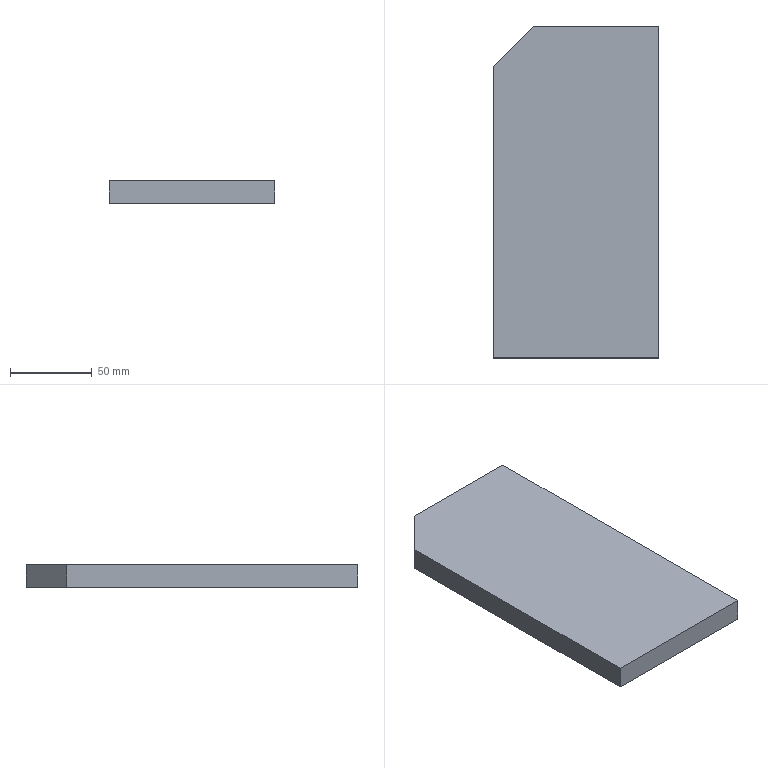Part | SolidWorks | features Chamfer 1, Extrusion 1 | 1 solid | 7 faces | box 101.6 x 203.2 x 14 mm | volume 284657 mm3 | plane 7
STEP:
#1=CARTESIAN_POINT('',(0.,178.2,7.));
#2=VERTEX_POINT('',#1);
#3=CARTESIAN_POINT('',(0.,0.,7.));
#4=VERTEX_POINT('',#3);
#5=CARTESIAN_POINT('',(0.,0.,7.));
#6=DIRECTION('',(0.,-1.,0.));
#7=VECTOR('',#6,1000.);
#8=LINE('',#5,#7);
#9=EDGE_CURVE('',#2,#4,#8,.T.);
#10=ORIENTED_EDGE('',*,*,#9,.F.);
#11=CARTESIAN_POINT('',(0.,178.2,-7.));
#12=VERTEX_POINT('',#11);
#13=CARTESIAN_POINT('',(0.,178.2,7.));
#14=DIRECTION('',(0.,0.,-1.));
#15=VECTOR('',#14,1000.);
#16=LINE('',#13,#15);
#17=EDGE_CURVE('',#2,#12,#16,.T.);
#18=ORIENTED_EDGE('',*,*,#17,.T.);
#19=CARTESIAN_POINT('',(0.,0.,-7.));
#20=VERTEX_POINT('',#19);
#21=CARTESIAN_POINT('',(0.,0.,-7.));
#22=DIRECTION('',(0.,-1.,0.));
#23=VECTOR('',#22,1000.);
#24=LINE('',#21,#23);
#25=EDGE_CURVE('',#12,#20,#24,.T.);
#26=ORIENTED_EDGE('',*,*,#25,.T.);
#27=CARTESIAN_POINT('',(0.,0.,7.));
#28=DIRECTION('',(0.,0.,-1.));
#29=VECTOR('',#28,1000.);
#30=LINE('',#27,#29);
#31=EDGE_CURVE('',#4,#20,#30,.T.);
#32=ORIENTED_EDGE('',*,*,#31,.F.);
#33=EDGE_LOOP('',(#10,#18,#26,#32));
#34=FACE_OUTER_BOUND('',#33,.T.);
#35=CARTESIAN_POINT('',(0.,0.,7.));
#36=DIRECTION('',(1.,0.,0.));
#37=DIRECTION('',(0.,0.,-1.));
#38=AXIS2_PLACEMENT_3D('',#35,#36,#37);
#39=PLANE('',#38);
#40=ADVANCED_FACE('',(#34),#39,.F.);
#41=CARTESIAN_POINT('',(101.6,0.,-7.));
#42=VERTEX_POINT('',#41);
#43=CARTESIAN_POINT('',(0.,0.,-7.));
#44=DIRECTION('',(1.,0.,0.));
#45=VECTOR('',#44,1000.);
#46=LINE('',#43,#45);
#47=EDGE_CURVE('',#20,#42,#46,.T.);
#48=ORIENTED_EDGE('',*,*,#47,.T.);
#49=CARTESIAN_POINT('',(101.6,0.,7.));
#50=VERTEX_POINT('',#49);
#51=CARTESIAN_POINT('',(101.6,0.,7.));
#52=DIRECTION('',(0.,0.,-1.));
#53=VECTOR('',#52,1000.);
#54=LINE('',#51,#53);
#55=EDGE_CURVE('',#50,#42,#54,.T.);
#56=ORIENTED_EDGE('',*,*,#55,.F.);
#57=CARTESIAN_POINT('',(0.,0.,7.));
#58=DIRECTION('',(1.,0.,0.));
#59=VECTOR('',#58,1000.);
#60=LINE('',#57,#59);
#61=EDGE_CURVE('',#4,#50,#60,.T.);
#62=ORIENTED_EDGE('',*,*,#61,.F.);
#63=ORIENTED_EDGE('',*,*,#31,.T.);
#64=EDGE_LOOP('',(#48,#56,#62,#63));
#65=FACE_OUTER_BOUND('',#64,.T.);
#66=CARTESIAN_POINT('',(0.,0.,7.));
#67=DIRECTION('',(0.,1.,0.));
#68=DIRECTION('',(0.,0.,1.));
#69=AXIS2_PLACEMENT_3D('',#66,#67,#68);
#70=PLANE('',#69);
#71=ADVANCED_FACE('',(#65),#70,.F.);
#72=CARTESIAN_POINT('',(101.6,203.2,-7.));
#73=VERTEX_POINT('',#72);
#74=CARTESIAN_POINT('',(101.6,0.,-7.));
#75=DIRECTION('',(0.,1.,0.));
#76=VECTOR('',#75,1000.);
#77=LINE('',#74,#76);
#78=EDGE_CURVE('',#42,#73,#77,.T.);
#79=ORIENTED_EDGE('',*,*,#78,.T.);
#80=CARTESIAN_POINT('',(101.6,203.2,7.));
#81=VERTEX_POINT('',#80);
#82=CARTESIAN_POINT('',(101.6,203.2,7.));
#83=DIRECTION('',(0.,0.,-1.));
#84=VECTOR('',#83,1000.);
#85=LINE('',#82,#84);
#86=EDGE_CURVE('',#81,#73,#85,.T.);
#87=ORIENTED_EDGE('',*,*,#86,.F.);
#88=CARTESIAN_POINT('',(101.6,0.,7.));
#89=DIRECTION('',(0.,1.,0.));
#90=VECTOR('',#89,1000.);
#91=LINE('',#88,#90);
#92=EDGE_CURVE('',#50,#81,#91,.T.);
#93=ORIENTED_EDGE('',*,*,#92,.F.);
#94=ORIENTED_EDGE('',*,*,#55,.T.);
#95=EDGE_LOOP('',(#79,#87,#93,#94));
#96=FACE_OUTER_BOUND('',#95,.T.);
#97=CARTESIAN_POINT('',(101.6,0.,7.));
#98=DIRECTION('',(-1.,0.,0.));
#99=DIRECTION('',(0.,0.,1.));
#100=AXIS2_PLACEMENT_3D('',#97,#98,#99);
#101=PLANE('',#100);
#102=ADVANCED_FACE('',(#96),#101,.F.);
#103=CARTESIAN_POINT('',(25.,203.2,-7.));
#104=VERTEX_POINT('',#103);
#105=CARTESIAN_POINT('',(0.,203.2,-7.));
#106=DIRECTION('',(-1.,0.,0.));
#107=VECTOR('',#106,1000.);
#108=LINE('',#105,#107);
#109=EDGE_CURVE('',#73,#104,#108,.T.);
#110=ORIENTED_EDGE('',*,*,#109,.T.);
#111=CARTESIAN_POINT('',(25.,203.2,7.));
#112=VERTEX_POINT('',#111);
#113=CARTESIAN_POINT('',(25.,203.2,7.));
#114=DIRECTION('',(0.,0.,1.));
#115=VECTOR('',#114,1000.);
#116=LINE('',#113,#115);
#117=EDGE_CURVE('',#104,#112,#116,.T.);
#118=ORIENTED_EDGE('',*,*,#117,.T.);
#119=CARTESIAN_POINT('',(0.,203.2,7.));
#120=DIRECTION('',(-1.,0.,0.));
#121=VECTOR('',#120,1000.);
#122=LINE('',#119,#121);
#123=EDGE_CURVE('',#81,#112,#122,.T.);
#124=ORIENTED_EDGE('',*,*,#123,.F.);
#125=ORIENTED_EDGE('',*,*,#86,.T.);
#126=EDGE_LOOP('',(#110,#118,#124,#125));
#127=FACE_OUTER_BOUND('',#126,.T.);
#128=CARTESIAN_POINT('',(0.,203.2,7.));
#129=DIRECTION('',(0.,-1.,0.));
#130=DIRECTION('',(0.,0.,-1.));
#131=AXIS2_PLACEMENT_3D('',#128,#129,#130);
#132=PLANE('',#131);
#133=ADVANCED_FACE('',(#127),#132,.F.);
#134=ORIENTED_EDGE('',*,*,#123,.T.);
#135=CARTESIAN_POINT('',(0.,178.2,7.));
#136=DIRECTION('',(-0.7071,-0.7071,0.));
#137=VECTOR('',#136,1000.);
#138=LINE('',#135,#137);
#139=EDGE_CURVE('',#112,#2,#138,.T.);
#140=ORIENTED_EDGE('',*,*,#139,.T.);
#141=ORIENTED_EDGE('',*,*,#9,.T.);
#142=ORIENTED_EDGE('',*,*,#61,.T.);
#143=ORIENTED_EDGE('',*,*,#92,.T.);
#144=EDGE_LOOP('',(#134,#140,#141,#142,#143));
#145=FACE_OUTER_BOUND('',#144,.T.);
#146=CARTESIAN_POINT('',(0.,203.2,7.));
#147=DIRECTION('',(0.,0.,-1.));
#148=DIRECTION('',(-1.,0.,0.));
#149=AXIS2_PLACEMENT_3D('',#146,#147,#148);
#150=PLANE('',#149);
#151=ADVANCED_FACE('',(#145),#150,.F.);
#152=ORIENTED_EDGE('',*,*,#25,.F.);
#153=CARTESIAN_POINT('',(12.5,190.7,-7.));
#154=DIRECTION('',(0.7071,0.7071,0.));
#155=VECTOR('',#154,1000.);
#156=LINE('',#153,#155);
#157=EDGE_CURVE('',#12,#104,#156,.T.);
#158=ORIENTED_EDGE('',*,*,#157,.T.);
#159=ORIENTED_EDGE('',*,*,#109,.F.);
#160=ORIENTED_EDGE('',*,*,#78,.F.);
#161=ORIENTED_EDGE('',*,*,#47,.F.);
#162=EDGE_LOOP('',(#152,#158,#159,#160,#161));
#163=FACE_OUTER_BOUND('',#162,.T.);
#164=CARTESIAN_POINT('',(0.,203.2,-7.));
#165=DIRECTION('',(0.,0.,-1.));
#166=DIRECTION('',(-1.,0.,0.));
#167=AXIS2_PLACEMENT_3D('',#164,#165,#166);
#168=PLANE('',#167);
#169=ADVANCED_FACE('',(#163),#168,.T.);
#170=ORIENTED_EDGE('',*,*,#139,.F.);
#171=ORIENTED_EDGE('',*,*,#117,.F.);
#172=ORIENTED_EDGE('',*,*,#157,.F.);
#173=ORIENTED_EDGE('',*,*,#17,.F.);
#174=EDGE_LOOP('',(#170,#171,#172,#173));
#175=FACE_OUTER_BOUND('',#174,.T.);
#176=CARTESIAN_POINT('',(0.,178.2,7.));
#177=DIRECTION('',(0.7071,-0.7071,0.));
#178=DIRECTION('',(0.7071,0.7071,0.));
#179=AXIS2_PLACEMENT_3D('',#176,#177,#178);
#180=PLANE('',#179);
#181=ADVANCED_FACE('',(#175),#180,.F.);
#182=CLOSED_SHELL('',(#40,#71,#102,#133,#151,#169,#181));
#183=MANIFOLD_SOLID_BREP('',#182);
#184=CARTESIAN_POINT('',(0.,0.,0.));
#185=DIRECTION('',(0.,0.,1.));
#186=DIRECTION('',(1.,0.,0.));
#187=AXIS2_PLACEMENT_3D('',#184,#185,#186);
#188=(LENGTH_UNIT()NAMED_UNIT(*)SI_UNIT(.MILLI.,.METRE.));
#189=UNCERTAINTY_MEASURE_WITH_UNIT(LENGTH_MEASURE(0.00001),#188,'','');
#190=(NAMED_UNIT(*)PLANE_ANGLE_UNIT()SI_UNIT($,.RADIAN.));
#191=(NAMED_UNIT(*)SI_UNIT($,.STERADIAN.)SOLID_ANGLE_UNIT());
#192=(GEOMETRIC_REPRESENTATION_CONTEXT(3)GLOBAL_UNCERTAINTY_ASSIGNED_CONTEXT((#189))GLOBAL_UNIT_ASSIGNED_CONTEXT((#188,#190,#191))REPRESENTATION_CONTEXT('',''));
#193=ADVANCED_BREP_SHAPE_REPRESENTATION('',(#183,#187),#192);